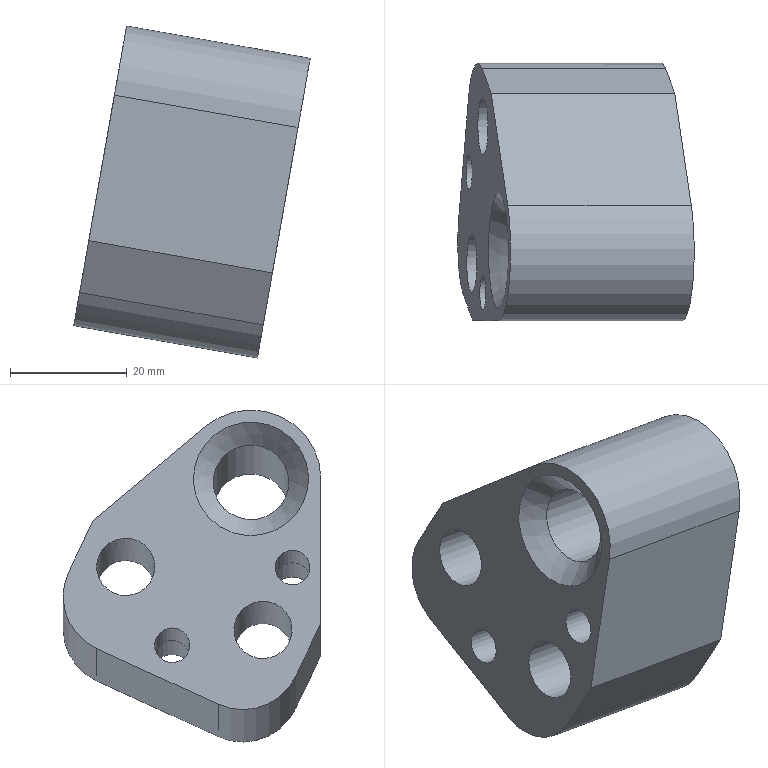Part | NX | features solid 2 | 1 solid | 24 faces | box 40.585 x 44.256 x 57 mm | volume 39763 mm3 | cylinder 12 | plane 11 | cone 1 | commonest cylinder face diameters 6 x2 8 x2 10 x2 14 x2 20 x2 13 x1
STEP:
#1=CARTESIAN_POINT('',(336.773,155.77,-17.405));
#2=VERTEX_POINT('',#1);
#3=CARTESIAN_POINT('',(337.067,159.395,-15.74));
#4=DIRECTION('',(0.9848,0.,-0.1736));
#5=DIRECTION('',(-0.07339,-0.9063,-0.4162));
#6=AXIS2_PLACEMENT_3D('',#3,#4,#5);
#7=CIRCLE('',#6,4.);
#8=EDGE_CURVE('',#2,#2,#7,.F.);
#9=ORIENTED_EDGE('',*,*,#8,.T.);
#10=EDGE_LOOP('',(#9));
#11=FACE_BOUND('',#10,.T.);
#12=CARTESIAN_POINT('',(338.336,170.332,-8.544));
#13=VERTEX_POINT('',#12);
#14=CARTESIAN_POINT('',(339.437,167.373,-2.296));
#15=DIRECTION('',(-0.9848,0.,0.1736));
#16=DIRECTION('',(-0.1574,0.4226,-0.8925));
#17=AXIS2_PLACEMENT_3D('',#14,#15,#16);
#18=CIRCLE('',#17,7.);
#19=EDGE_CURVE('',#13,#13,#18,.T.);
#20=ORIENTED_EDGE('',*,*,#19,.T.);
#21=EDGE_LOOP('',(#20));
#22=FACE_BOUND('',#21,.T.);
#23=CARTESIAN_POINT('',(336.428,146.768,-19.365));
#24=VERTEX_POINT('',#23);
#25=CARTESIAN_POINT('',(337.529,143.809,-13.117));
#26=DIRECTION('',(-0.9848,0.,0.1736));
#27=DIRECTION('',(-0.1574,0.4226,-0.8925));
#28=AXIS2_PLACEMENT_3D('',#25,#26,#27);
#29=CIRCLE('',#28,7.);
#30=EDGE_CURVE('',#24,#24,#29,.T.);
#31=ORIENTED_EDGE('',*,*,#30,.T.);
#32=EDGE_LOOP('',(#31));
#33=FACE_BOUND('',#32,.T.);
#34=CARTESIAN_POINT('',(341.626,139.98,10.116));
#35=VERTEX_POINT('',#34);
#36=CARTESIAN_POINT('',(342.103,145.871,12.821));
#37=DIRECTION('',(0.9848,0.,-0.1736));
#38=DIRECTION('',(-0.07339,-0.9063,-0.4162));
#39=AXIS2_PLACEMENT_3D('',#36,#37,#38);
#40=CIRCLE('',#39,6.5);
#41=EDGE_CURVE('',#35,#35,#40,.T.);
#42=ORIENTED_EDGE('',*,*,#41,.F.);
#43=EDGE_LOOP('',(#42));
#44=FACE_BOUND('',#43,.T.);
#45=CARTESIAN_POINT('',(339.274,177.19,-3.221));
#46=VERTEX_POINT('',#45);
#47=CARTESIAN_POINT('',(336.967,172.353,-16.309));
#48=VERTEX_POINT('',#47);
#49=CARTESIAN_POINT('',(338.54,168.127,-7.383));
#50=DIRECTION('',(-0.9848,0.,0.1736));
#51=DIRECTION('',(-0.1574,0.4226,-0.8925));
#52=AXIS2_PLACEMENT_3D('',#49,#50,#51);
#53=CIRCLE('',#52,10.);
#54=EDGE_CURVE('',#46,#48,#53,.T.);
#55=ORIENTED_EDGE('',*,*,#54,.F.);
#56=CARTESIAN_POINT('',(340.848,172.964,5.704));
#57=VERTEX_POINT('',#56);
#58=CARTESIAN_POINT('',(340.848,172.964,5.704));
#59=DIRECTION('',(-0.1574,0.4226,-0.8925));
#60=VECTOR('',#59,1000.);
#61=LINE('',#58,#60);
#62=EDGE_CURVE('',#57,#46,#61,.T.);
#63=ORIENTED_EDGE('',*,*,#62,.F.);
#64=CARTESIAN_POINT('',(343.693,153.629,21.838));
#65=VERTEX_POINT('',#64);
#66=CARTESIAN_POINT('',(343.693,153.629,21.838));
#67=DIRECTION('',(-0.1123,0.763,-0.6366));
#68=VECTOR('',#67,1000.);
#69=LINE('',#66,#68);
#70=EDGE_CURVE('',#65,#57,#69,.T.);
#71=ORIENTED_EDGE('',*,*,#70,.F.);
#72=CARTESIAN_POINT('',(342.093,133.871,12.765));
#73=VERTEX_POINT('',#72);
#74=CARTESIAN_POINT('',(342.103,145.871,12.821));
#75=DIRECTION('',(-0.9848,0.,0.1736));
#76=DIRECTION('',(-0.1574,0.4226,-0.8925));
#77=AXIS2_PLACEMENT_3D('',#74,#75,#76);
#78=CIRCLE('',#77,12.);
#79=EDGE_CURVE('',#73,#65,#78,.T.);
#80=ORIENTED_EDGE('',*,*,#79,.F.);
#81=CARTESIAN_POINT('',(337.692,133.993,-12.192));
#82=VERTEX_POINT('',#81);
#83=CARTESIAN_POINT('',(342.093,133.871,12.765));
#84=DIRECTION('',(-0.1736,0.004789,-0.9848));
#85=VECTOR('',#84,1000.);
#86=LINE('',#83,#85);
#87=EDGE_CURVE('',#73,#82,#86,.T.);
#88=ORIENTED_EDGE('',*,*,#87,.T.);
#89=CARTESIAN_POINT('',(336.119,138.219,-21.118));
#90=VERTEX_POINT('',#89);
#91=CARTESIAN_POINT('',(337.692,133.993,-12.192));
#92=DIRECTION('',(-0.1574,0.4226,-0.8925));
#93=VECTOR('',#92,1000.);
#94=LINE('',#91,#93);
#95=EDGE_CURVE('',#82,#90,#94,.T.);
#96=ORIENTED_EDGE('',*,*,#95,.T.);
#97=CARTESIAN_POINT('',(335.279,151.508,-25.881));
#98=VERTEX_POINT('',#97);
#99=CARTESIAN_POINT('',(336.852,147.282,-16.956));
#100=DIRECTION('',(-0.9848,0.,0.1736));
#101=DIRECTION('',(-0.1574,0.4226,-0.8925));
#102=AXIS2_PLACEMENT_3D('',#99,#100,#101);
#103=CIRCLE('',#102,10.);
#104=EDGE_CURVE('',#98,#90,#103,.T.);
#105=ORIENTED_EDGE('',*,*,#104,.F.);
#106=CARTESIAN_POINT('',(335.279,151.508,-25.881));
#107=DIRECTION('',(0.07339,0.9063,0.4162));
#108=VECTOR('',#107,1000.);
#109=LINE('',#106,#108);
#110=EDGE_CURVE('',#98,#48,#109,.T.);
#111=ORIENTED_EDGE('',*,*,#110,.T.);
#112=EDGE_LOOP('',(#55,#63,#71,#80,#88,#96,#105,#111));
#113=FACE_BOUND('',#112,.T.);
#114=CARTESIAN_POINT('',(339.124,135.113,-4.072));
#115=VERTEX_POINT('',#114);
#116=CARTESIAN_POINT('',(339.418,138.738,-2.407));
#117=DIRECTION('',(0.9848,0.,-0.1736));
#118=DIRECTION('',(-0.07339,-0.9063,-0.4162));
#119=AXIS2_PLACEMENT_3D('',#116,#117,#118);
#120=CIRCLE('',#119,4.);
#121=EDGE_CURVE('',#115,#115,#120,.F.);
#122=ORIENTED_EDGE('',*,*,#121,.T.);
#123=EDGE_LOOP('',(#122));
#124=FACE_BOUND('',#123,.T.);
#125=CARTESIAN_POINT('',(338.54,168.127,-7.383));
#126=DIRECTION('',(0.9848,0.,-0.1736));
#127=DIRECTION('',(0.07339,0.9063,0.4162));
#128=AXIS2_PLACEMENT_3D('',#125,#126,#127);
#129=PLANE('',#128);
#130=ADVANCED_FACE('',(#11,#22,#33,#44,#113,#124),#129,.T.);
#131=CARTESIAN_POINT('',(307.137,169.487,-1.202));
#132=VERTEX_POINT('',#131);
#133=CARTESIAN_POINT('',(307.923,167.373,3.26));
#134=DIRECTION('',(-0.9848,0.,0.1736));
#135=DIRECTION('',(-0.1574,0.4226,-0.8925));
#136=AXIS2_PLACEMENT_3D('',#133,#134,#135);
#137=CIRCLE('',#136,5.);
#138=EDGE_CURVE('',#132,#132,#137,.T.);
#139=ORIENTED_EDGE('',*,*,#138,.T.);
#140=EDGE_LOOP('',(#139));
#141=FACE_BOUND('',#140,.T.);
#142=CARTESIAN_POINT('',(329.956,171.905,1.521));
#143=VERTEX_POINT('',#142);
#144=CARTESIAN_POINT('',(329.589,167.373,-0.5599));
#145=DIRECTION('',(-0.9848,0.,0.1736));
#146=DIRECTION('',(0.07339,0.9063,0.4162));
#147=AXIS2_PLACEMENT_3D('',#144,#145,#146);
#148=CIRCLE('',#147,5.);
#149=EDGE_CURVE('',#143,#143,#148,.T.);
#150=ORIENTED_EDGE('',*,*,#149,.F.);
#151=EDGE_LOOP('',(#150));
#152=FACE_BOUND('',#151,.T.);
#153=CARTESIAN_POINT('',(339.437,167.373,-2.296));
#154=DIRECTION('',(-0.9848,0.,0.1736));
#155=DIRECTION('',(-0.07339,-0.9063,-0.4162));
#156=AXIS2_PLACEMENT_3D('',#153,#154,#155);
#157=CYLINDRICAL_SURFACE('',#156,5.);
#158=ADVANCED_FACE('',(#141,#152),#157,.F.);
#159=CARTESIAN_POINT('',(305.229,145.923,-12.023));
#160=VERTEX_POINT('',#159);
#161=CARTESIAN_POINT('',(306.015,143.809,-7.561));
#162=DIRECTION('',(-0.9848,0.,0.1736));
#163=DIRECTION('',(-0.1574,0.4226,-0.8925));
#164=AXIS2_PLACEMENT_3D('',#161,#162,#163);
#165=CIRCLE('',#164,5.);
#166=EDGE_CURVE('',#160,#160,#165,.T.);
#167=ORIENTED_EDGE('',*,*,#166,.T.);
#168=EDGE_LOOP('',(#167));
#169=FACE_BOUND('',#168,.T.);
#170=CARTESIAN_POINT('',(328.048,148.341,-9.3));
#171=VERTEX_POINT('',#170);
#172=CARTESIAN_POINT('',(327.681,143.809,-11.381));
#173=DIRECTION('',(-0.9848,0.,0.1736));
#174=DIRECTION('',(0.07339,0.9063,0.4162));
#175=AXIS2_PLACEMENT_3D('',#172,#173,#174);
#176=CIRCLE('',#175,5.);
#177=EDGE_CURVE('',#171,#171,#176,.T.);
#178=ORIENTED_EDGE('',*,*,#177,.F.);
#179=EDGE_LOOP('',(#178));
#180=FACE_BOUND('',#179,.T.);
#181=CARTESIAN_POINT('',(337.529,143.809,-13.117));
#182=DIRECTION('',(-0.9848,0.,0.1736));
#183=DIRECTION('',(-0.07339,-0.9063,-0.4162));
#184=AXIS2_PLACEMENT_3D('',#181,#182,#183);
#185=CYLINDRICAL_SURFACE('',#184,5.);
#186=ADVANCED_FACE('',(#169,#180),#185,.F.);
#187=CARTESIAN_POINT('',(307.432,140.006,0.4721));
#188=VERTEX_POINT('',#187);
#189=CARTESIAN_POINT('',(307.904,138.738,3.15));
#190=DIRECTION('',(-0.9848,0.,0.1736));
#191=DIRECTION('',(-0.1574,0.4226,-0.8925));
#192=AXIS2_PLACEMENT_3D('',#189,#190,#191);
#193=CIRCLE('',#192,3.);
#194=EDGE_CURVE('',#188,#188,#193,.T.);
#195=ORIENTED_EDGE('',*,*,#194,.F.);
#196=EDGE_LOOP('',(#195));
#197=FACE_BOUND('',#196,.T.);
#198=ORIENTED_EDGE('',*,*,#166,.F.);
#199=EDGE_LOOP('',(#198));
#200=FACE_BOUND('',#199,.T.);
#201=CARTESIAN_POINT('',(311.316,154.844,22.499));
#202=VERTEX_POINT('',#201);
#203=CARTESIAN_POINT('',(310.589,145.871,18.378));
#204=DIRECTION('',(-0.9848,0.,0.1736));
#205=DIRECTION('',(0.07339,0.9063,0.4162));
#206=AXIS2_PLACEMENT_3D('',#203,#204,#205);
#207=CIRCLE('',#206,9.9);
#208=EDGE_CURVE('',#202,#202,#207,.T.);
#209=ORIENTED_EDGE('',*,*,#208,.F.);
#210=EDGE_LOOP('',(#209));
#211=FACE_BOUND('',#210,.T.);
#212=CARTESIAN_POINT('',(307.76,177.19,2.335));
#213=VERTEX_POINT('',#212);
#214=CARTESIAN_POINT('',(305.453,172.353,-10.752));
#215=VERTEX_POINT('',#214);
#216=CARTESIAN_POINT('',(307.027,168.127,-1.827));
#217=DIRECTION('',(-0.9848,0.,0.1736));
#218=DIRECTION('',(-0.1574,0.4226,-0.8925));
#219=AXIS2_PLACEMENT_3D('',#216,#217,#218);
#220=CIRCLE('',#219,10.);
#221=EDGE_CURVE('',#213,#215,#220,.T.);
#222=ORIENTED_EDGE('',*,*,#221,.T.);
#223=CARTESIAN_POINT('',(303.765,151.508,-20.325));
#224=VERTEX_POINT('',#223);
#225=CARTESIAN_POINT('',(303.765,151.508,-20.325));
#226=DIRECTION('',(0.07339,0.9063,0.4162));
#227=VECTOR('',#226,1000.);
#228=LINE('',#225,#227);
#229=EDGE_CURVE('',#224,#215,#228,.T.);
#230=ORIENTED_EDGE('',*,*,#229,.F.);
#231=CARTESIAN_POINT('',(304.605,138.219,-15.561));
#232=VERTEX_POINT('',#231);
#233=CARTESIAN_POINT('',(305.339,147.282,-11.399));
#234=DIRECTION('',(-0.9848,0.,0.1736));
#235=DIRECTION('',(-0.1574,0.4226,-0.8925));
#236=AXIS2_PLACEMENT_3D('',#233,#234,#235);
#237=CIRCLE('',#236,10.);
#238=EDGE_CURVE('',#224,#232,#237,.T.);
#239=ORIENTED_EDGE('',*,*,#238,.T.);
#240=CARTESIAN_POINT('',(306.179,133.993,-6.636));
#241=VERTEX_POINT('',#240);
#242=CARTESIAN_POINT('',(306.179,133.993,-6.636));
#243=DIRECTION('',(-0.1574,0.4226,-0.8925));
#244=VECTOR('',#243,1000.);
#245=LINE('',#242,#244);
#246=EDGE_CURVE('',#241,#232,#245,.T.);
#247=ORIENTED_EDGE('',*,*,#246,.F.);
#248=CARTESIAN_POINT('',(310.579,133.871,18.322));
#249=VERTEX_POINT('',#248);
#250=CARTESIAN_POINT('',(310.579,133.871,18.322));
#251=DIRECTION('',(-0.1736,0.004789,-0.9848));
#252=VECTOR('',#251,1000.);
#253=LINE('',#250,#252);
#254=EDGE_CURVE('',#249,#241,#253,.T.);
#255=ORIENTED_EDGE('',*,*,#254,.F.);
#256=CARTESIAN_POINT('',(312.179,153.629,27.395));
#257=VERTEX_POINT('',#256);
#258=CARTESIAN_POINT('',(310.589,145.871,18.378));
#259=DIRECTION('',(-0.9848,0.,0.1736));
#260=DIRECTION('',(-0.1574,0.4226,-0.8925));
#261=AXIS2_PLACEMENT_3D('',#258,#259,#260);
#262=CIRCLE('',#261,12.);
#263=EDGE_CURVE('',#249,#257,#262,.T.);
#264=ORIENTED_EDGE('',*,*,#263,.T.);
#265=CARTESIAN_POINT('',(309.334,172.964,11.261));
#266=VERTEX_POINT('',#265);
#267=CARTESIAN_POINT('',(312.179,153.629,27.395));
#268=DIRECTION('',(-0.1123,0.763,-0.6366));
#269=VECTOR('',#268,1000.);
#270=LINE('',#267,#269);
#271=EDGE_CURVE('',#257,#266,#270,.T.);
#272=ORIENTED_EDGE('',*,*,#271,.T.);
#273=CARTESIAN_POINT('',(309.334,172.964,11.261));
#274=DIRECTION('',(-0.1574,0.4226,-0.8925));
#275=VECTOR('',#274,1000.);
#276=LINE('',#273,#275);
#277=EDGE_CURVE('',#266,#213,#276,.T.);
#278=ORIENTED_EDGE('',*,*,#277,.T.);
#279=EDGE_LOOP('',(#222,#230,#239,#247,#255,#264,#272,#278));
#280=FACE_BOUND('',#279,.T.);
#281=ORIENTED_EDGE('',*,*,#138,.F.);
#282=EDGE_LOOP('',(#281));
#283=FACE_BOUND('',#282,.T.);
#284=CARTESIAN_POINT('',(305.081,160.663,-12.861));
#285=VERTEX_POINT('',#284);
#286=CARTESIAN_POINT('',(305.553,159.395,-10.183));
#287=DIRECTION('',(-0.9848,0.,0.1736));
#288=DIRECTION('',(-0.1574,0.4226,-0.8925));
#289=AXIS2_PLACEMENT_3D('',#286,#287,#288);
#290=CIRCLE('',#289,3.);
#291=EDGE_CURVE('',#285,#285,#290,.T.);
#292=ORIENTED_EDGE('',*,*,#291,.F.);
#293=EDGE_LOOP('',(#292));
#294=FACE_BOUND('',#293,.T.);
#295=CARTESIAN_POINT('',(307.027,168.127,-1.827));
#296=DIRECTION('',(0.9848,0.,-0.1736));
#297=DIRECTION('',(0.07339,0.9063,0.4162));
#298=AXIS2_PLACEMENT_3D('',#295,#296,#297);
#299=PLANE('',#298);
#300=ADVANCED_FACE('',(#197,#200,#211,#280,#283,#294),#299,.F.);
#301=ORIENTED_EDGE('',*,*,#221,.F.);
#302=CARTESIAN_POINT('',(339.274,177.19,-3.221));
#303=DIRECTION('',(-0.9848,0.,0.1736));
#304=VECTOR('',#303,1000.);
#305=LINE('',#302,#304);
#306=EDGE_CURVE('',#46,#213,#305,.T.);
#307=ORIENTED_EDGE('',*,*,#306,.F.);
#308=ORIENTED_EDGE('',*,*,#54,.T.);
#309=CARTESIAN_POINT('',(336.967,172.353,-16.309));
#310=DIRECTION('',(-0.9848,0.,0.1736));
#311=VECTOR('',#310,1000.);
#312=LINE('',#309,#311);
#313=EDGE_CURVE('',#48,#215,#312,.T.);
#314=ORIENTED_EDGE('',*,*,#313,.T.);
#315=EDGE_LOOP('',(#301,#307,#308,#314));
#316=FACE_BOUND('',#315,.T.);
#317=CARTESIAN_POINT('',(338.54,168.127,-7.383));
#318=DIRECTION('',(-0.9848,0.,0.1736));
#319=DIRECTION('',(-0.07339,-0.9063,-0.4162));
#320=AXIS2_PLACEMENT_3D('',#317,#318,#319);
#321=CYLINDRICAL_SURFACE('',#320,10.);
#322=ADVANCED_FACE('',(#316),#321,.T.);
#323=ORIENTED_EDGE('',*,*,#229,.T.);
#324=ORIENTED_EDGE('',*,*,#313,.F.);
#325=ORIENTED_EDGE('',*,*,#110,.F.);
#326=CARTESIAN_POINT('',(335.279,151.508,-25.881));
#327=DIRECTION('',(-0.9848,0.,0.1736));
#328=VECTOR('',#327,1000.);
#329=LINE('',#326,#328);
#330=EDGE_CURVE('',#98,#224,#329,.T.);
#331=ORIENTED_EDGE('',*,*,#330,.T.);
#332=EDGE_LOOP('',(#323,#324,#325,#331));
#333=FACE_BOUND('',#332,.T.);
#334=CARTESIAN_POINT('',(335.279,151.508,-25.881));
#335=DIRECTION('',(-0.1574,0.4226,-0.8925));
#336=DIRECTION('',(0.07339,0.9063,0.4162));
#337=AXIS2_PLACEMENT_3D('',#334,#335,#336);
#338=PLANE('',#337);
#339=ADVANCED_FACE('',(#333),#338,.T.);
#340=ORIENTED_EDGE('',*,*,#238,.F.);
#341=ORIENTED_EDGE('',*,*,#330,.F.);
#342=ORIENTED_EDGE('',*,*,#104,.T.);
#343=CARTESIAN_POINT('',(336.119,138.219,-21.118));
#344=DIRECTION('',(-0.9848,0.,0.1736));
#345=VECTOR('',#344,1000.);
#346=LINE('',#343,#345);
#347=EDGE_CURVE('',#90,#232,#346,.T.);
#348=ORIENTED_EDGE('',*,*,#347,.T.);
#349=EDGE_LOOP('',(#340,#341,#342,#348));
#350=FACE_BOUND('',#349,.T.);
#351=CARTESIAN_POINT('',(336.852,147.282,-16.956));
#352=DIRECTION('',(-0.9848,0.,0.1736));
#353=DIRECTION('',(-0.07339,-0.9063,-0.4162));
#354=AXIS2_PLACEMENT_3D('',#351,#352,#353);
#355=CYLINDRICAL_SURFACE('',#354,10.);
#356=ADVANCED_FACE('',(#350),#355,.T.);
#357=ORIENTED_EDGE('',*,*,#246,.T.);
#358=ORIENTED_EDGE('',*,*,#347,.F.);
#359=ORIENTED_EDGE('',*,*,#95,.F.);
#360=CARTESIAN_POINT('',(337.692,133.993,-12.192));
#361=DIRECTION('',(-0.9848,0.,0.1736));
#362=VECTOR('',#361,1000.);
#363=LINE('',#360,#362);
#364=EDGE_CURVE('',#82,#241,#363,.T.);
#365=ORIENTED_EDGE('',*,*,#364,.T.);
#366=EDGE_LOOP('',(#357,#358,#359,#365));
#367=FACE_BOUND('',#366,.T.);
#368=CARTESIAN_POINT('',(337.692,133.993,-12.192));
#369=DIRECTION('',(-0.07339,-0.9063,-0.4162));
#370=DIRECTION('',(0.9848,0.,-0.1736));
#371=AXIS2_PLACEMENT_3D('',#368,#369,#370);
#372=PLANE('',#371);
#373=ADVANCED_FACE('',(#367),#372,.T.);
#374=ORIENTED_EDGE('',*,*,#254,.T.);
#375=ORIENTED_EDGE('',*,*,#364,.F.);
#376=ORIENTED_EDGE('',*,*,#87,.F.);
#377=CARTESIAN_POINT('',(342.093,133.871,12.765));
#378=DIRECTION('',(-0.9848,0.,0.1736));
#379=VECTOR('',#378,1000.);
#380=LINE('',#377,#379);
#381=EDGE_CURVE('',#73,#249,#380,.T.);
#382=ORIENTED_EDGE('',*,*,#381,.T.);
#383=EDGE_LOOP('',(#374,#375,#376,#382));
#384=FACE_BOUND('',#383,.T.);
#385=CARTESIAN_POINT('',(342.093,133.871,12.765));
#386=DIRECTION('',(-0.0008317,-1.,-0.004717));
#387=DIRECTION('',(-0.1736,0.004789,-0.9848));
#388=AXIS2_PLACEMENT_3D('',#385,#386,#387);
#389=PLANE('',#388);
#390=ADVANCED_FACE('',(#384),#389,.T.);
#391=ORIENTED_EDGE('',*,*,#263,.F.);
#392=ORIENTED_EDGE('',*,*,#381,.F.);
#393=ORIENTED_EDGE('',*,*,#79,.T.);
#394=CARTESIAN_POINT('',(343.693,153.629,21.838));
#395=DIRECTION('',(-0.9848,0.,0.1736));
#396=VECTOR('',#395,1000.);
#397=LINE('',#394,#396);
#398=EDGE_CURVE('',#65,#257,#397,.T.);
#399=ORIENTED_EDGE('',*,*,#398,.T.);
#400=EDGE_LOOP('',(#391,#392,#393,#399));
#401=FACE_BOUND('',#400,.T.);
#402=CARTESIAN_POINT('',(342.103,145.871,12.821));
#403=DIRECTION('',(-0.9848,0.,0.1736));
#404=DIRECTION('',(-0.07339,-0.9063,-0.4162));
#405=AXIS2_PLACEMENT_3D('',#402,#403,#404);
#406=CYLINDRICAL_SURFACE('',#405,12.);
#407=ADVANCED_FACE('',(#401),#406,.T.);
#408=ORIENTED_EDGE('',*,*,#271,.F.);
#409=ORIENTED_EDGE('',*,*,#398,.F.);
#410=ORIENTED_EDGE('',*,*,#70,.T.);
#411=CARTESIAN_POINT('',(340.848,172.964,5.704));
#412=DIRECTION('',(-0.9848,0.,0.1736));
#413=VECTOR('',#412,1000.);
#414=LINE('',#411,#413);
#415=EDGE_CURVE('',#57,#266,#414,.T.);
#416=ORIENTED_EDGE('',*,*,#415,.T.);
#417=EDGE_LOOP('',(#408,#409,#410,#416));
#418=FACE_BOUND('',#417,.T.);
#419=CARTESIAN_POINT('',(343.693,153.629,21.838));
#420=DIRECTION('',(-0.1325,-0.6464,-0.7514));
#421=DIRECTION('',(-0.1123,0.763,-0.6366));
#422=AXIS2_PLACEMENT_3D('',#419,#420,#421);
#423=PLANE('',#422);
#424=ADVANCED_FACE('',(#418),#423,.F.);
#425=ORIENTED_EDGE('',*,*,#277,.F.);
#426=ORIENTED_EDGE('',*,*,#415,.F.);
#427=ORIENTED_EDGE('',*,*,#62,.T.);
#428=ORIENTED_EDGE('',*,*,#306,.T.);
#429=EDGE_LOOP('',(#425,#426,#427,#428));
#430=FACE_BOUND('',#429,.T.);
#431=CARTESIAN_POINT('',(340.848,172.964,5.704));
#432=DIRECTION('',(-0.07339,-0.9063,-0.4162));
#433=DIRECTION('',(-0.1574,0.4226,-0.8925));
#434=AXIS2_PLACEMENT_3D('',#431,#432,#433);
#435=PLANE('',#434);
#436=ADVANCED_FACE('',(#430),#435,.F.);
#437=ORIENTED_EDGE('',*,*,#41,.T.);
#438=EDGE_LOOP('',(#437));
#439=FACE_BOUND('',#438,.T.);
#440=CARTESIAN_POINT('',(313.46,139.98,15.083));
#441=VERTEX_POINT('',#440);
#442=CARTESIAN_POINT('',(313.938,145.871,17.788));
#443=DIRECTION('',(-0.9848,0.,0.1736));
#444=DIRECTION('',(-0.07339,-0.9063,-0.4162));
#445=AXIS2_PLACEMENT_3D('',#442,#443,#444);
#446=CIRCLE('',#445,6.5);
#447=EDGE_CURVE('',#441,#441,#446,.T.);
#448=ORIENTED_EDGE('',*,*,#447,.T.);
#449=EDGE_LOOP('',(#448));
#450=FACE_BOUND('',#449,.T.);
#451=CARTESIAN_POINT('',(342.103,145.871,12.821));
#452=DIRECTION('',(-0.9848,0.,0.1736));
#453=DIRECTION('',(-0.07339,-0.9063,-0.4162));
#454=AXIS2_PLACEMENT_3D('',#451,#452,#453);
#455=CYLINDRICAL_SURFACE('',#454,6.5);
#456=ADVANCED_FACE('',(#439,#450),#455,.F.);
#457=ORIENTED_EDGE('',*,*,#208,.T.);
#458=EDGE_LOOP('',(#457));
#459=FACE_BOUND('',#458,.T.);
#460=ORIENTED_EDGE('',*,*,#447,.F.);
#461=EDGE_LOOP('',(#460));
#462=FACE_BOUND('',#461,.T.);
#463=CARTESIAN_POINT('',(313.938,145.871,17.788));
#464=DIRECTION('',(-0.9848,0.,0.1736));
#465=DIRECTION('',(-0.07339,-0.9063,-0.4162));
#466=AXIS2_PLACEMENT_3D('',#463,#464,#465);
#467=CONICAL_SURFACE('',#466,6.5,0.7854);
#468=ADVANCED_FACE('',(#459,#462),#467,.F.);
#469=CARTESIAN_POINT('',(319.25,140.006,-1.612));
#470=VERTEX_POINT('',#469);
#471=CARTESIAN_POINT('',(319.722,138.738,1.066));
#472=DIRECTION('',(-0.9848,0.,0.1736));
#473=DIRECTION('',(-0.1574,0.4226,-0.8925));
#474=AXIS2_PLACEMENT_3D('',#471,#472,#473);
#475=CIRCLE('',#474,3.);
#476=EDGE_CURVE('',#470,#470,#475,.T.);
#477=ORIENTED_EDGE('',*,*,#476,.F.);
#478=EDGE_LOOP('',(#477));
#479=FACE_BOUND('',#478,.T.);
#480=ORIENTED_EDGE('',*,*,#194,.T.);
#481=EDGE_LOOP('',(#480));
#482=FACE_BOUND('',#481,.T.);
#483=CARTESIAN_POINT('',(339.418,138.738,-2.407));
#484=DIRECTION('',(-0.9848,0.,0.1736));
#485=DIRECTION('',(-0.07339,-0.9063,-0.4162));
#486=AXIS2_PLACEMENT_3D('',#483,#484,#485);
#487=CYLINDRICAL_SURFACE('',#486,3.);
#488=ADVANCED_FACE('',(#479,#482),#487,.F.);
#489=CARTESIAN_POINT('',(316.899,160.663,-14.944));
#490=VERTEX_POINT('',#489);
#491=CARTESIAN_POINT('',(317.371,159.395,-12.267));
#492=DIRECTION('',(-0.9848,0.,0.1736));
#493=DIRECTION('',(-0.1574,0.4226,-0.8925));
#494=AXIS2_PLACEMENT_3D('',#491,#492,#493);
#495=CIRCLE('',#494,3.);
#496=EDGE_CURVE('',#490,#490,#495,.T.);
#497=ORIENTED_EDGE('',*,*,#496,.F.);
#498=EDGE_LOOP('',(#497));
#499=FACE_BOUND('',#498,.T.);
#500=ORIENTED_EDGE('',*,*,#291,.T.);
#501=EDGE_LOOP('',(#500));
#502=FACE_BOUND('',#501,.T.);
#503=CARTESIAN_POINT('',(337.067,159.395,-15.74));
#504=DIRECTION('',(-0.9848,0.,0.1736));
#505=DIRECTION('',(-0.07339,-0.9063,-0.4162));
#506=AXIS2_PLACEMENT_3D('',#503,#504,#505);
#507=CYLINDRICAL_SURFACE('',#506,3.);
#508=ADVANCED_FACE('',(#499,#502),#507,.F.);
#509=CARTESIAN_POINT('',(326.58,146.768,-17.629));
#510=VERTEX_POINT('',#509);
#511=CARTESIAN_POINT('',(327.681,143.809,-11.381));
#512=DIRECTION('',(-0.9848,0.,0.1736));
#513=DIRECTION('',(-0.1574,0.4226,-0.8925));
#514=AXIS2_PLACEMENT_3D('',#511,#512,#513);
#515=CIRCLE('',#514,7.);
#516=EDGE_CURVE('',#510,#510,#515,.T.);
#517=ORIENTED_EDGE('',*,*,#516,.T.);
#518=EDGE_LOOP('',(#517));
#519=FACE_BOUND('',#518,.T.);
#520=ORIENTED_EDGE('',*,*,#30,.F.);
#521=EDGE_LOOP('',(#520));
#522=FACE_BOUND('',#521,.T.);
#523=CARTESIAN_POINT('',(327.681,143.809,-11.381));
#524=DIRECTION('',(0.9848,0.,-0.1736));
#525=DIRECTION('',(0.07339,0.9063,0.4162));
#526=AXIS2_PLACEMENT_3D('',#523,#524,#525);
#527=CYLINDRICAL_SURFACE('',#526,7.);
#528=ADVANCED_FACE('',(#519,#522),#527,.F.);
#529=ORIENTED_EDGE('',*,*,#177,.T.);
#530=EDGE_LOOP('',(#529));
#531=FACE_BOUND('',#530,.T.);
#532=ORIENTED_EDGE('',*,*,#516,.F.);
#533=EDGE_LOOP('',(#532));
#534=FACE_BOUND('',#533,.T.);
#535=CARTESIAN_POINT('',(327.681,143.809,-11.381));
#536=DIRECTION('',(0.9848,0.,-0.1736));
#537=DIRECTION('',(0.07339,0.9063,0.4162));
#538=AXIS2_PLACEMENT_3D('',#535,#536,#537);
#539=PLANE('',#538);
#540=ADVANCED_FACE('',(#531,#534),#539,.T.);
#541=CARTESIAN_POINT('',(328.488,170.332,-6.808));
#542=VERTEX_POINT('',#541);
#543=CARTESIAN_POINT('',(329.589,167.373,-0.5599));
#544=DIRECTION('',(-0.9848,0.,0.1736));
#545=DIRECTION('',(-0.1574,0.4226,-0.8925));
#546=AXIS2_PLACEMENT_3D('',#543,#544,#545);
#547=CIRCLE('',#546,7.);
#548=EDGE_CURVE('',#542,#542,#547,.T.);
#549=ORIENTED_EDGE('',*,*,#548,.T.);
#550=EDGE_LOOP('',(#549));
#551=FACE_BOUND('',#550,.T.);
#552=ORIENTED_EDGE('',*,*,#19,.F.);
#553=EDGE_LOOP('',(#552));
#554=FACE_BOUND('',#553,.T.);
#555=CARTESIAN_POINT('',(329.589,167.373,-0.5599));
#556=DIRECTION('',(0.9848,0.,-0.1736));
#557=DIRECTION('',(0.07339,0.9063,0.4162));
#558=AXIS2_PLACEMENT_3D('',#555,#556,#557);
#559=CYLINDRICAL_SURFACE('',#558,7.);
#560=ADVANCED_FACE('',(#551,#554),#559,.F.);
#561=ORIENTED_EDGE('',*,*,#149,.T.);
#562=EDGE_LOOP('',(#561));
#563=FACE_BOUND('',#562,.T.);
#564=ORIENTED_EDGE('',*,*,#548,.F.);
#565=EDGE_LOOP('',(#564));
#566=FACE_BOUND('',#565,.T.);
#567=CARTESIAN_POINT('',(329.589,167.373,-0.5599));
#568=DIRECTION('',(0.9848,0.,-0.1736));
#569=DIRECTION('',(0.07339,0.9063,0.4162));
#570=AXIS2_PLACEMENT_3D('',#567,#568,#569);
#571=PLANE('',#570);
#572=ADVANCED_FACE('',(#563,#566),#571,.T.);
#573=CARTESIAN_POINT('',(317.077,155.77,-13.932));
#574=VERTEX_POINT('',#573);
#575=CARTESIAN_POINT('',(317.371,159.395,-12.267));
#576=DIRECTION('',(0.9848,0.,-0.1736));
#577=DIRECTION('',(-0.07339,-0.9063,-0.4162));
#578=AXIS2_PLACEMENT_3D('',#575,#576,#577);
#579=CIRCLE('',#578,4.);
#580=EDGE_CURVE('',#574,#574,#579,.F.);
#581=ORIENTED_EDGE('',*,*,#580,.F.);
#582=EDGE_LOOP('',(#581));
#583=FACE_BOUND('',#582,.T.);
#584=ORIENTED_EDGE('',*,*,#496,.T.);
#585=EDGE_LOOP('',(#584));
#586=FACE_BOUND('',#585,.T.);
#587=CARTESIAN_POINT('',(317.371,159.395,-12.267));
#588=DIRECTION('',(-0.9848,0.,0.1736));
#589=DIRECTION('',(-0.07339,-0.9063,-0.4162));
#590=AXIS2_PLACEMENT_3D('',#587,#588,#589);
#591=PLANE('',#590);
#592=ADVANCED_FACE('',(#583,#586),#591,.F.);
#593=ORIENTED_EDGE('',*,*,#580,.T.);
#594=EDGE_LOOP('',(#593));
#595=FACE_BOUND('',#594,.T.);
#596=ORIENTED_EDGE('',*,*,#8,.F.);
#597=EDGE_LOOP('',(#596));
#598=FACE_BOUND('',#597,.T.);
#599=CARTESIAN_POINT('',(337.067,159.395,-15.74));
#600=DIRECTION('',(-0.9848,0.,0.1736));
#601=DIRECTION('',(-0.07339,-0.9063,-0.4162));
#602=AXIS2_PLACEMENT_3D('',#599,#600,#601);
#603=CYLINDRICAL_SURFACE('',#602,4.);
#604=ADVANCED_FACE('',(#595,#598),#603,.F.);
#605=CARTESIAN_POINT('',(319.428,135.113,-0.5988));
#606=VERTEX_POINT('',#605);
#607=CARTESIAN_POINT('',(319.722,138.738,1.066));
#608=DIRECTION('',(0.9848,0.,-0.1736));
#609=DIRECTION('',(-0.07339,-0.9063,-0.4162));
#610=AXIS2_PLACEMENT_3D('',#607,#608,#609);
#611=CIRCLE('',#610,4.);
#612=EDGE_CURVE('',#606,#606,#611,.F.);
#613=ORIENTED_EDGE('',*,*,#612,.F.);
#614=EDGE_LOOP('',(#613));
#615=FACE_BOUND('',#614,.T.);
#616=ORIENTED_EDGE('',*,*,#476,.T.);
#617=EDGE_LOOP('',(#616));
#618=FACE_BOUND('',#617,.T.);
#619=CARTESIAN_POINT('',(319.722,138.738,1.066));
#620=DIRECTION('',(-0.9848,0.,0.1736));
#621=DIRECTION('',(-0.07339,-0.9063,-0.4162));
#622=AXIS2_PLACEMENT_3D('',#619,#620,#621);
#623=PLANE('',#622);
#624=ADVANCED_FACE('',(#615,#618),#623,.F.);
#625=ORIENTED_EDGE('',*,*,#612,.T.);
#626=EDGE_LOOP('',(#625));
#627=FACE_BOUND('',#626,.T.);
#628=ORIENTED_EDGE('',*,*,#121,.F.);
#629=EDGE_LOOP('',(#628));
#630=FACE_BOUND('',#629,.T.);
#631=CARTESIAN_POINT('',(339.418,138.738,-2.407));
#632=DIRECTION('',(-0.9848,0.,0.1736));
#633=DIRECTION('',(-0.07339,-0.9063,-0.4162));
#634=AXIS2_PLACEMENT_3D('',#631,#632,#633);
#635=CYLINDRICAL_SURFACE('',#634,4.);
#636=ADVANCED_FACE('',(#627,#630),#635,.F.);
#637=CLOSED_SHELL('',(#130,#158,#186,#300,#322,#339,#356,#373,#390,#407,#424,#436,#456,#468,#488,#508,#528,#540,#560,#572,#592,#604,#624,#636));
#638=MANIFOLD_SOLID_BREP('',#637);
#639=(LENGTH_UNIT()NAMED_UNIT(*)SI_UNIT(.MILLI.,.METRE.));
#640=UNCERTAINTY_MEASURE_WITH_UNIT(LENGTH_MEASURE(0.00001),#639,'','');
#641=(NAMED_UNIT(*)PLANE_ANGLE_UNIT()SI_UNIT($,.RADIAN.));
#642=(NAMED_UNIT(*)SI_UNIT($,.STERADIAN.)SOLID_ANGLE_UNIT());
#643=(GEOMETRIC_REPRESENTATION_CONTEXT(3)GLOBAL_UNCERTAINTY_ASSIGNED_CONTEXT((#640))GLOBAL_UNIT_ASSIGNED_CONTEXT((#639,#641,#642))REPRESENTATION_CONTEXT('',''));
#644=ADVANCED_BREP_SHAPE_REPRESENTATION('',(#638),#643);